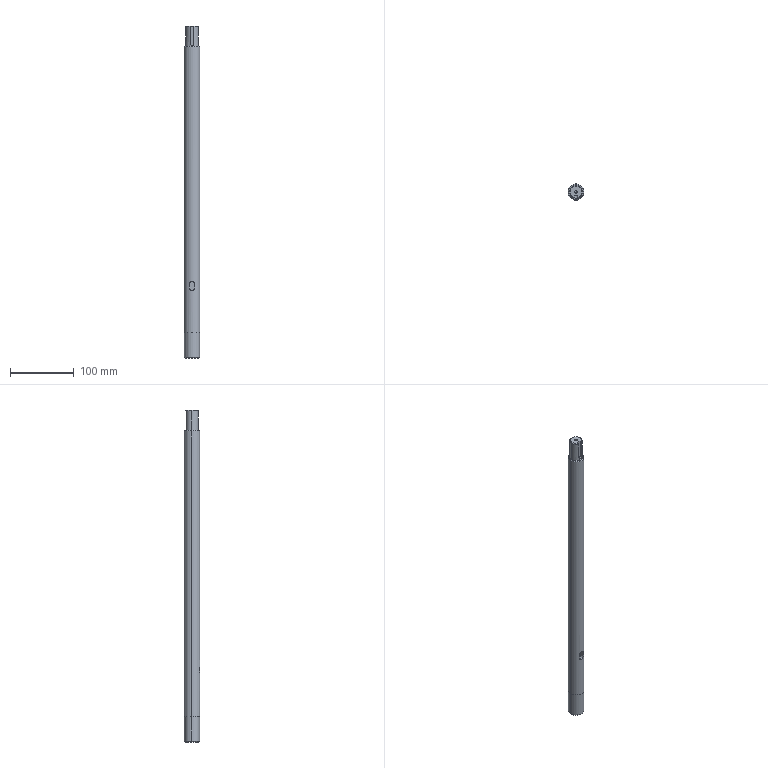Part | SolidWorks | features ICE 4, Chamfer 1, Extrusion 1, Fillet 1, HoleWzd 1 | 1 solid | 32 faces | box 25 x 25 x 522 mm | volume 247598 mm3 | cylinder 13 | plane 10 | cone 9 | commonest cylinder face diameters 8 x4 4.2 x2 20 x2 24 x2 25 x2 6 x1
STEP:
#1=CARTESIAN_POINT('',(-2.1,0.,244.6));
#2=VERTEX_POINT('',#1);
#3=CARTESIAN_POINT('',(2.1,0.,244.6));
#4=VERTEX_POINT('',#3);
#5=CARTESIAN_POINT('',(0.,0.,244.6));
#6=DIRECTION('',(0.,0.,1.));
#7=DIRECTION('',(1.,0.,0.));
#8=AXIS2_PLACEMENT_3D('',#5,#6,#7);
#9=CIRCLE('',#8,2.1);
#10=EDGE_CURVE('',#2,#4,#9,.T.);
#11=ORIENTED_EDGE('',*,*,#10,.F.);
#12=CARTESIAN_POINT('',(-2.1,0.,257.));
#13=VERTEX_POINT('',#12);
#14=CARTESIAN_POINT('',(-2.1,0.,257.));
#15=DIRECTION('',(0.,0.,1.));
#16=VECTOR('',#15,1000.);
#17=LINE('',#14,#16);
#18=EDGE_CURVE('',#2,#13,#17,.T.);
#19=ORIENTED_EDGE('',*,*,#18,.T.);
#20=CARTESIAN_POINT('',(2.1,0.,257.));
#21=VERTEX_POINT('',#20);
#22=CARTESIAN_POINT('',(0.,0.,257.));
#23=DIRECTION('',(0.,0.,1.));
#24=DIRECTION('',(1.,0.,0.));
#25=AXIS2_PLACEMENT_3D('',#22,#23,#24);
#26=CIRCLE('',#25,2.1);
#27=EDGE_CURVE('',#13,#21,#26,.T.);
#28=ORIENTED_EDGE('',*,*,#27,.T.);
#29=CARTESIAN_POINT('',(2.1,0.,257.));
#30=DIRECTION('',(0.,0.,1.));
#31=VECTOR('',#30,1000.);
#32=LINE('',#29,#31);
#33=EDGE_CURVE('',#4,#21,#32,.T.);
#34=ORIENTED_EDGE('',*,*,#33,.F.);
#35=EDGE_LOOP('',(#11,#19,#28,#34));
#36=FACE_OUTER_BOUND('',#35,.T.);
#37=CARTESIAN_POINT('',(0.,0.,257.));
#38=DIRECTION('',(0.,0.,1.));
#39=DIRECTION('',(1.,0.,0.));
#40=AXIS2_PLACEMENT_3D('',#37,#38,#39);
#41=CYLINDRICAL_SURFACE('',#40,2.1);
#42=ADVANCED_FACE('',(#36),#41,.F.);
#43=CARTESIAN_POINT('',(0.,0.,243.338));
#44=VERTEX_POINT('',#43);
#45=CARTESIAN_POINT('',(2.1,0.,244.6));
#46=DIRECTION('',(0.8572,0.,0.515));
#47=VECTOR('',#46,1000.);
#48=LINE('',#45,#47);
#49=EDGE_CURVE('',#44,#4,#48,.T.);
#50=ORIENTED_EDGE('',*,*,#49,.F.);
#51=CARTESIAN_POINT('',(-2.1,0.,244.6));
#52=DIRECTION('',(-0.8572,0.,0.515));
#53=VECTOR('',#52,1000.);
#54=LINE('',#51,#53);
#55=EDGE_CURVE('',#44,#2,#54,.T.);
#56=ORIENTED_EDGE('',*,*,#55,.T.);
#57=ORIENTED_EDGE('',*,*,#10,.T.);
#58=EDGE_LOOP('',(#50,#56,#57));
#59=FACE_OUTER_BOUND('',#58,.T.);
#60=CARTESIAN_POINT('',(0.,0.,244.6));
#61=DIRECTION('',(0.,0.,1.));
#62=DIRECTION('',(1.,0.,0.));
#63=AXIS2_PLACEMENT_3D('',#60,#61,#62);
#64=CONICAL_SURFACE('',#63,2.1,1.03);
#65=ADVANCED_FACE('',(#59),#64,.F.);
#66=CARTESIAN_POINT('',(-11.,0.,-265.));
#67=VERTEX_POINT('',#66);
#68=CARTESIAN_POINT('',(11.,0.,-265.));
#69=VERTEX_POINT('',#68);
#70=CARTESIAN_POINT('',(0.,0.,-265.));
#71=DIRECTION('',(0.,0.,-1.));
#72=DIRECTION('',(-1.,0.,0.));
#73=AXIS2_PLACEMENT_3D('',#70,#71,#72);
#74=CIRCLE('',#73,11.);
#75=EDGE_CURVE('',#67,#69,#74,.T.);
#76=ORIENTED_EDGE('',*,*,#75,.F.);
#77=CARTESIAN_POINT('',(-12.,0.,-264.));
#78=VERTEX_POINT('',#77);
#79=CARTESIAN_POINT('',(-11.,0.,-265.));
#80=DIRECTION('',(-0.7071,0.,0.7071));
#81=VECTOR('',#80,1000.);
#82=LINE('',#79,#81);
#83=EDGE_CURVE('',#67,#78,#82,.T.);
#84=ORIENTED_EDGE('',*,*,#83,.T.);
#85=CARTESIAN_POINT('',(12.,0.,-264.));
#86=VERTEX_POINT('',#85);
#87=CARTESIAN_POINT('',(0.,0.,-264.));
#88=DIRECTION('',(0.,0.,1.));
#89=DIRECTION('',(-1.,0.,0.));
#90=AXIS2_PLACEMENT_3D('',#87,#88,#89);
#91=CIRCLE('',#90,12.);
#92=EDGE_CURVE('',#86,#78,#91,.T.);
#93=ORIENTED_EDGE('',*,*,#92,.F.);
#94=CARTESIAN_POINT('',(11.,0.,-265.));
#95=DIRECTION('',(0.7071,0.,0.7071));
#96=VECTOR('',#95,1000.);
#97=LINE('',#94,#96);
#98=EDGE_CURVE('',#69,#86,#97,.T.);
#99=ORIENTED_EDGE('',*,*,#98,.F.);
#100=EDGE_LOOP('',(#76,#84,#93,#99));
#101=FACE_OUTER_BOUND('',#100,.T.);
#102=CARTESIAN_POINT('',(0.,0.,-265.));
#103=DIRECTION('',(0.,0.,1.));
#104=DIRECTION('',(1.,0.,0.));
#105=AXIS2_PLACEMENT_3D('',#102,#103,#104);
#106=CONICAL_SURFACE('',#105,11.,0.7854);
#107=ADVANCED_FACE('',(#101),#106,.T.);
#108=CARTESIAN_POINT('',(11.5,0.,225.));
#109=VERTEX_POINT('',#108);
#110=CARTESIAN_POINT('',(-11.5,0.,225.));
#111=VERTEX_POINT('',#110);
#112=CARTESIAN_POINT('',(0.,0.,225.));
#113=DIRECTION('',(0.,0.,1.));
#114=DIRECTION('',(1.,0.,0.));
#115=AXIS2_PLACEMENT_3D('',#112,#113,#114);
#116=CIRCLE('',#115,11.5);
#117=EDGE_CURVE('',#109,#111,#116,.T.);
#118=ORIENTED_EDGE('',*,*,#117,.F.);
#119=CARTESIAN_POINT('',(12.5,0.,224.));
#120=VERTEX_POINT('',#119);
#121=CARTESIAN_POINT('',(11.5,0.,225.));
#122=DIRECTION('',(0.7071,0.,-0.7071));
#123=VECTOR('',#122,1000.);
#124=LINE('',#121,#123);
#125=EDGE_CURVE('',#109,#120,#124,.T.);
#126=ORIENTED_EDGE('',*,*,#125,.T.);
#127=CARTESIAN_POINT('',(-12.5,0.,224.));
#128=VERTEX_POINT('',#127);
#129=CARTESIAN_POINT('',(0.,0.,224.));
#130=DIRECTION('',(0.,0.,-1.));
#131=DIRECTION('',(1.,0.,0.));
#132=AXIS2_PLACEMENT_3D('',#129,#130,#131);
#133=CIRCLE('',#132,12.5);
#134=EDGE_CURVE('',#128,#120,#133,.T.);
#135=ORIENTED_EDGE('',*,*,#134,.F.);
#136=CARTESIAN_POINT('',(-11.5,0.,225.));
#137=DIRECTION('',(-0.7071,0.,-0.7071));
#138=VECTOR('',#137,1000.);
#139=LINE('',#136,#138);
#140=EDGE_CURVE('',#111,#128,#139,.T.);
#141=ORIENTED_EDGE('',*,*,#140,.F.);
#142=EDGE_LOOP('',(#118,#126,#135,#141));
#143=FACE_OUTER_BOUND('',#142,.T.);
#144=CARTESIAN_POINT('',(0.,0.,225.));
#145=DIRECTION('',(0.,0.,-1.));
#146=DIRECTION('',(-1.,0.,0.));
#147=AXIS2_PLACEMENT_3D('',#144,#145,#146);
#148=CONICAL_SURFACE('',#147,11.5,0.7854);
#149=ADVANCED_FACE('',(#143),#148,.T.);
#150=CARTESIAN_POINT('',(9.,0.,257.));
#151=VERTEX_POINT('',#150);
#152=CARTESIAN_POINT('',(-9.,0.,257.));
#153=VERTEX_POINT('',#152);
#154=CARTESIAN_POINT('',(0.,0.,257.));
#155=DIRECTION('',(0.,0.,1.));
#156=DIRECTION('',(1.,0.,0.));
#157=AXIS2_PLACEMENT_3D('',#154,#155,#156);
#158=CIRCLE('',#157,9.);
#159=EDGE_CURVE('',#151,#153,#158,.T.);
#160=ORIENTED_EDGE('',*,*,#159,.F.);
#161=CARTESIAN_POINT('',(10.,0.,256.));
#162=VERTEX_POINT('',#161);
#163=CARTESIAN_POINT('',(9.,0.,257.));
#164=DIRECTION('',(0.7071,0.,-0.7071));
#165=VECTOR('',#164,1000.);
#166=LINE('',#163,#165);
#167=EDGE_CURVE('',#151,#162,#166,.T.);
#168=ORIENTED_EDGE('',*,*,#167,.T.);
#169=CARTESIAN_POINT('',(-10.,0.,256.));
#170=VERTEX_POINT('',#169);
#171=CARTESIAN_POINT('',(0.,0.,256.));
#172=DIRECTION('',(0.,0.,-1.));
#173=DIRECTION('',(1.,0.,0.));
#174=AXIS2_PLACEMENT_3D('',#171,#172,#173);
#175=CIRCLE('',#174,10.);
#176=EDGE_CURVE('',#170,#162,#175,.T.);
#177=ORIENTED_EDGE('',*,*,#176,.F.);
#178=CARTESIAN_POINT('',(-9.,0.,257.));
#179=DIRECTION('',(-0.7071,0.,-0.7071));
#180=VECTOR('',#179,1000.);
#181=LINE('',#178,#180);
#182=EDGE_CURVE('',#153,#170,#181,.T.);
#183=ORIENTED_EDGE('',*,*,#182,.F.);
#184=EDGE_LOOP('',(#160,#168,#177,#183));
#185=FACE_OUTER_BOUND('',#184,.T.);
#186=CARTESIAN_POINT('',(0.,0.,257.));
#187=DIRECTION('',(0.,0.,-1.));
#188=DIRECTION('',(-1.,0.,0.));
#189=AXIS2_PLACEMENT_3D('',#186,#187,#188);
#190=CONICAL_SURFACE('',#189,9.,0.7854);
#191=ADVANCED_FACE('',(#185),#190,.T.);
#192=CARTESIAN_POINT('',(-3.,-8.485,257.));
#193=VERTEX_POINT('',#192);
#194=CARTESIAN_POINT('',(0.,0.,257.));
#195=DIRECTION('',(0.,0.,1.));
#196=DIRECTION('',(1.,0.,0.));
#197=AXIS2_PLACEMENT_3D('',#194,#195,#196);
#198=CIRCLE('',#197,9.);
#199=EDGE_CURVE('',#153,#193,#198,.T.);
#200=ORIENTED_EDGE('',*,*,#199,.F.);
#201=ORIENTED_EDGE('',*,*,#182,.T.);
#202=CARTESIAN_POINT('',(-3.,-9.539,256.));
#203=VERTEX_POINT('',#202);
#204=CARTESIAN_POINT('',(0.,0.,256.));
#205=DIRECTION('',(0.,0.,-1.));
#206=DIRECTION('',(1.,0.,0.));
#207=AXIS2_PLACEMENT_3D('',#204,#205,#206);
#208=CIRCLE('',#207,10.);
#209=EDGE_CURVE('',#203,#170,#208,.T.);
#210=ORIENTED_EDGE('',*,*,#209,.F.);
#211=CARTESIAN_POINT('',(-3.,-8.485,257.));
#212=CARTESIAN_POINT('',(-3.,-8.838,256.668));
#213=CARTESIAN_POINT('',(-3.,-9.189,256.334));
#214=CARTESIAN_POINT('',(-3.,-9.539,256.));
#215=B_SPLINE_CURVE_WITH_KNOTS('',3,(#211,#212,#213,#214),.UNSPECIFIED.,.F.,.F.,(4,4),(0.,0.001453),.UNSPECIFIED.);
#216=EDGE_CURVE('',#193,#203,#215,.T.);
#217=ORIENTED_EDGE('',*,*,#216,.F.);
#218=EDGE_LOOP('',(#200,#201,#210,#217));
#219=FACE_OUTER_BOUND('',#218,.T.);
#220=CARTESIAN_POINT('',(0.,0.,257.));
#221=DIRECTION('',(0.,0.,-1.));
#222=DIRECTION('',(-1.,0.,0.));
#223=AXIS2_PLACEMENT_3D('',#220,#221,#222);
#224=CONICAL_SURFACE('',#223,9.,0.7854);
#225=ADVANCED_FACE('',(#219),#224,.T.);
#226=ORIENTED_EDGE('',*,*,#92,.T.);
#227=CARTESIAN_POINT('',(-12.,0.,-225.));
#228=VERTEX_POINT('',#227);
#229=CARTESIAN_POINT('',(-12.,0.,-265.));
#230=DIRECTION('',(0.,0.,1.));
#231=VECTOR('',#230,1000.);
#232=LINE('',#229,#231);
#233=EDGE_CURVE('',#78,#228,#232,.T.);
#234=ORIENTED_EDGE('',*,*,#233,.T.);
#235=CARTESIAN_POINT('',(12.,0.,-225.));
#236=VERTEX_POINT('',#235);
#237=CARTESIAN_POINT('',(0.,0.,-225.));
#238=DIRECTION('',(0.,0.,-1.));
#239=DIRECTION('',(-1.,0.,0.));
#240=AXIS2_PLACEMENT_3D('',#237,#238,#239);
#241=CIRCLE('',#240,12.);
#242=EDGE_CURVE('',#228,#236,#241,.T.);
#243=ORIENTED_EDGE('',*,*,#242,.T.);
#244=CARTESIAN_POINT('',(12.,0.,-265.));
#245=DIRECTION('',(0.,0.,1.));
#246=VECTOR('',#245,1000.);
#247=LINE('',#244,#246);
#248=EDGE_CURVE('',#86,#236,#247,.T.);
#249=ORIENTED_EDGE('',*,*,#248,.F.);
#250=EDGE_LOOP('',(#226,#234,#243,#249));
#251=FACE_OUTER_BOUND('',#250,.T.);
#252=CARTESIAN_POINT('',(0.,0.,-265.));
#253=DIRECTION('',(0.,0.,1.));
#254=DIRECTION('',(1.,0.,0.));
#255=AXIS2_PLACEMENT_3D('',#252,#253,#254);
#256=CYLINDRICAL_SURFACE('',#255,12.);
#257=ADVANCED_FACE('',(#251),#256,.T.);
#258=ORIENTED_EDGE('',*,*,#176,.T.);
#259=CARTESIAN_POINT('',(10.,0.,225.));
#260=VERTEX_POINT('',#259);
#261=CARTESIAN_POINT('',(10.,0.,257.));
#262=DIRECTION('',(0.,0.,-1.));
#263=VECTOR('',#262,1000.);
#264=LINE('',#261,#263);
#265=EDGE_CURVE('',#162,#260,#264,.T.);
#266=ORIENTED_EDGE('',*,*,#265,.T.);
#267=CARTESIAN_POINT('',(-10.,0.,225.));
#268=VERTEX_POINT('',#267);
#269=CARTESIAN_POINT('',(0.,0.,225.));
#270=DIRECTION('',(0.,0.,1.));
#271=DIRECTION('',(1.,0.,0.));
#272=AXIS2_PLACEMENT_3D('',#269,#270,#271);
#273=CIRCLE('',#272,10.);
#274=EDGE_CURVE('',#260,#268,#273,.T.);
#275=ORIENTED_EDGE('',*,*,#274,.T.);
#276=CARTESIAN_POINT('',(-10.,0.,257.));
#277=DIRECTION('',(0.,0.,-1.));
#278=VECTOR('',#277,1000.);
#279=LINE('',#276,#278);
#280=EDGE_CURVE('',#170,#268,#279,.T.);
#281=ORIENTED_EDGE('',*,*,#280,.F.);
#282=EDGE_LOOP('',(#258,#266,#275,#281));
#283=FACE_OUTER_BOUND('',#282,.T.);
#284=CARTESIAN_POINT('',(0.,0.,257.));
#285=DIRECTION('',(0.,0.,-1.));
#286=DIRECTION('',(-1.,0.,0.));
#287=AXIS2_PLACEMENT_3D('',#284,#285,#286);
#288=CYLINDRICAL_SURFACE('',#287,10.);
#289=ADVANCED_FACE('',(#283),#288,.T.);
#290=ORIENTED_EDGE('',*,*,#134,.T.);
#291=CARTESIAN_POINT('',(12.5,0.,-225.));
#292=VERTEX_POINT('',#291);
#293=CARTESIAN_POINT('',(12.5,0.,225.));
#294=DIRECTION('',(0.,0.,-1.));
#295=VECTOR('',#294,1000.);
#296=LINE('',#293,#295);
#297=EDGE_CURVE('',#120,#292,#296,.T.);
#298=ORIENTED_EDGE('',*,*,#297,.T.);
#299=CARTESIAN_POINT('',(-12.5,0.,-225.));
#300=VERTEX_POINT('',#299);
#301=CARTESIAN_POINT('',(0.,0.,-225.));
#302=DIRECTION('',(0.,0.,1.));
#303=DIRECTION('',(1.,0.,0.));
#304=AXIS2_PLACEMENT_3D('',#301,#302,#303);
#305=CIRCLE('',#304,12.5);
#306=EDGE_CURVE('',#292,#300,#305,.T.);
#307=ORIENTED_EDGE('',*,*,#306,.T.);
#308=CARTESIAN_POINT('',(-12.5,0.,225.));
#309=DIRECTION('',(0.,0.,-1.));
#310=VECTOR('',#309,1000.);
#311=LINE('',#308,#310);
#312=EDGE_CURVE('',#128,#300,#311,.T.);
#313=ORIENTED_EDGE('',*,*,#312,.F.);
#314=EDGE_LOOP('',(#290,#298,#307,#313));
#315=FACE_OUTER_BOUND('',#314,.T.);
#316=CARTESIAN_POINT('',(0.,0.,225.));
#317=DIRECTION('',(0.,0.,-1.));
#318=DIRECTION('',(-1.,0.,0.));
#319=AXIS2_PLACEMENT_3D('',#316,#317,#318);
#320=CYLINDRICAL_SURFACE('',#319,12.5);
#321=ADVANCED_FACE('',(#315),#320,.T.);
#322=ORIENTED_EDGE('',*,*,#297,.F.);
#323=CARTESIAN_POINT('',(0.,0.,224.));
#324=DIRECTION('',(0.,0.,-1.));
#325=DIRECTION('',(1.,0.,0.));
#326=AXIS2_PLACEMENT_3D('',#323,#324,#325);
#327=CIRCLE('',#326,12.5);
#328=EDGE_CURVE('',#120,#128,#327,.T.);
#329=ORIENTED_EDGE('',*,*,#328,.T.);
#330=ORIENTED_EDGE('',*,*,#312,.T.);
#331=CARTESIAN_POINT('',(0.,0.,-225.));
#332=DIRECTION('',(0.,0.,1.));
#333=DIRECTION('',(1.,0.,0.));
#334=AXIS2_PLACEMENT_3D('',#331,#332,#333);
#335=CIRCLE('',#334,12.5);
#336=EDGE_CURVE('',#300,#292,#335,.T.);
#337=ORIENTED_EDGE('',*,*,#336,.T.);
#338=EDGE_LOOP('',(#322,#329,#330,#337));
#339=FACE_OUTER_BOUND('',#338,.T.);
#340=CARTESIAN_POINT('',(4.,-11.843,-155.));
#341=VERTEX_POINT('',#340);
#342=CARTESIAN_POINT('',(0.,-12.5,-159.));
#343=VERTEX_POINT('',#342);
#344=CARTESIAN_POINT('',(4.,-11.843,-155.));
#345=CARTESIAN_POINT('',(4.,-11.843,-155.266));
#346=CARTESIAN_POINT('',(3.974,-11.852,-155.527));
#347=CARTESIAN_POINT('',(3.871,-11.886,-156.04));
#348=CARTESIAN_POINT('',(3.794,-11.911,-156.295));
#349=CARTESIAN_POINT('',(3.592,-11.973,-156.779));
#350=CARTESIAN_POINT('',(3.47,-12.01,-157.007));
#351=CARTESIAN_POINT('',(3.18,-12.09,-157.441));
#352=CARTESIAN_POINT('',(3.012,-12.133,-157.644));
#353=CARTESIAN_POINT('',(2.646,-12.218,-158.011));
#354=CARTESIAN_POINT('',(2.446,-12.26,-158.176));
#355=CARTESIAN_POINT('',(2.01,-12.339,-158.468));
#356=CARTESIAN_POINT('',(1.78,-12.375,-158.591));
#357=CARTESIAN_POINT('',(1.3,-12.435,-158.792));
#358=CARTESIAN_POINT('',(1.047,-12.459,-158.87));
#359=CARTESIAN_POINT('',(0.5285,-12.492,-158.974));
#360=CARTESIAN_POINT('',(0.266,-12.5,-159.));
#361=CARTESIAN_POINT('',(0.,-12.5,-159.));
#362=B_SPLINE_CURVE_WITH_KNOTS('',3,(#344,#345,#346,#347,#348,#349,#350,#351,#352,#353,#354,#355,#356,#357,#358,#359,#360,#361),.UNSPECIFIED.,.F.,.F.,(4,2,2,2,2,2,2,2,4),(0.,0.0007863,0.001573,0.002359,0.003145,0.003931,0.004718,0.005504,0.00629),.UNSPECIFIED.);
#363=EDGE_CURVE('',#341,#343,#362,.T.);
#364=ORIENTED_EDGE('',*,*,#363,.T.);
#365=CARTESIAN_POINT('',(-4.,-11.843,-155.));
#366=VERTEX_POINT('',#365);
#367=CARTESIAN_POINT('',(0.,-12.5,-159.));
#368=CARTESIAN_POINT('',(-0.266,-12.5,-159.));
#369=CARTESIAN_POINT('',(-0.5272,-12.492,-158.974));
#370=CARTESIAN_POINT('',(-1.041,-12.459,-158.871));
#371=CARTESIAN_POINT('',(-1.296,-12.435,-158.793));
#372=CARTESIAN_POINT('',(-1.779,-12.375,-158.592));
#373=CARTESIAN_POINT('',(-2.008,-12.34,-158.469));
#374=CARTESIAN_POINT('',(-2.441,-12.261,-158.179));
#375=CARTESIAN_POINT('',(-2.645,-12.218,-158.012));
#376=CARTESIAN_POINT('',(-3.011,-12.133,-157.646));
#377=CARTESIAN_POINT('',(-3.176,-12.091,-157.446));
#378=CARTESIAN_POINT('',(-3.469,-12.01,-157.009));
#379=CARTESIAN_POINT('',(-3.592,-11.973,-156.78));
#380=CARTESIAN_POINT('',(-3.792,-11.911,-156.3));
#381=CARTESIAN_POINT('',(-3.87,-11.886,-156.046));
#382=CARTESIAN_POINT('',(-3.974,-11.852,-155.528));
#383=CARTESIAN_POINT('',(-4.,-11.843,-155.266));
#384=CARTESIAN_POINT('',(-4.,-11.843,-155.));
#385=B_SPLINE_CURVE_WITH_KNOTS('',3,(#367,#368,#369,#370,#371,#372,#373,#374,#375,#376,#377,#378,#379,#380,#381,#382,#383,#384),.UNSPECIFIED.,.F.,.F.,(4,2,2,2,2,2,2,2,4),(0.,0.0007863,0.001573,0.002359,0.003145,0.003932,0.004718,0.005504,0.00629),.UNSPECIFIED.);
#386=EDGE_CURVE('',#343,#366,#385,.T.);
#387=ORIENTED_EDGE('',*,*,#386,.T.);
#388=CARTESIAN_POINT('',(-4.,-11.843,-148.));
#389=VERTEX_POINT('',#388);
#390=CARTESIAN_POINT('',(-4.,-11.843,225.));
#391=DIRECTION('',(0.,0.,1.));
#392=VECTOR('',#391,1000.);
#393=LINE('',#390,#392);
#394=EDGE_CURVE('',#366,#389,#393,.T.);
#395=ORIENTED_EDGE('',*,*,#394,.T.);
#396=CARTESIAN_POINT('',(0.,-12.5,-144.));
#397=VERTEX_POINT('',#396);
#398=CARTESIAN_POINT('',(-4.,-11.843,-148.));
#399=CARTESIAN_POINT('',(-4.,-11.843,-147.734));
#400=CARTESIAN_POINT('',(-3.974,-11.852,-147.473));
#401=CARTESIAN_POINT('',(-3.871,-11.886,-146.96));
#402=CARTESIAN_POINT('',(-3.794,-11.911,-146.705));
#403=CARTESIAN_POINT('',(-3.592,-11.973,-146.221));
#404=CARTESIAN_POINT('',(-3.47,-12.01,-145.993));
#405=CARTESIAN_POINT('',(-3.18,-12.09,-145.559));
#406=CARTESIAN_POINT('',(-3.012,-12.133,-145.356));
#407=CARTESIAN_POINT('',(-2.646,-12.218,-144.989));
#408=CARTESIAN_POINT('',(-2.446,-12.26,-144.824));
#409=CARTESIAN_POINT('',(-2.01,-12.339,-144.532));
#410=CARTESIAN_POINT('',(-1.78,-12.375,-144.409));
#411=CARTESIAN_POINT('',(-1.3,-12.435,-144.208));
#412=CARTESIAN_POINT('',(-1.047,-12.459,-144.13));
#413=CARTESIAN_POINT('',(-0.5285,-12.492,-144.026));
#414=CARTESIAN_POINT('',(-0.266,-12.5,-144.));
#415=CARTESIAN_POINT('',(0.,-12.5,-144.));
#416=B_SPLINE_CURVE_WITH_KNOTS('',3,(#398,#399,#400,#401,#402,#403,#404,#405,#406,#407,#408,#409,#410,#411,#412,#413,#414,#415),.UNSPECIFIED.,.F.,.F.,(4,2,2,2,2,2,2,2,4),(0.,0.0007863,0.001573,0.002359,0.003145,0.003931,0.004718,0.005504,0.00629),.UNSPECIFIED.);
#417=EDGE_CURVE('',#389,#397,#416,.T.);
#418=ORIENTED_EDGE('',*,*,#417,.T.);
#419=CARTESIAN_POINT('',(4.,-11.843,-148.));
#420=VERTEX_POINT('',#419);
#421=CARTESIAN_POINT('',(0.,-12.5,-144.));
#422=CARTESIAN_POINT('',(0.266,-12.5,-144.));
#423=CARTESIAN_POINT('',(0.5272,-12.492,-144.026));
#424=CARTESIAN_POINT('',(1.041,-12.459,-144.129));
#425=CARTESIAN_POINT('',(1.296,-12.435,-144.207));
#426=CARTESIAN_POINT('',(1.779,-12.375,-144.408));
#427=CARTESIAN_POINT('',(2.008,-12.34,-144.531));
#428=CARTESIAN_POINT('',(2.441,-12.261,-144.821));
#429=CARTESIAN_POINT('',(2.645,-12.218,-144.988));
#430=CARTESIAN_POINT('',(3.011,-12.133,-145.354));
#431=CARTESIAN_POINT('',(3.176,-12.091,-145.554));
#432=CARTESIAN_POINT('',(3.469,-12.01,-145.991));
#433=CARTESIAN_POINT('',(3.592,-11.973,-146.22));
#434=CARTESIAN_POINT('',(3.792,-11.911,-146.7));
#435=CARTESIAN_POINT('',(3.87,-11.886,-146.954));
#436=CARTESIAN_POINT('',(3.974,-11.852,-147.472));
#437=CARTESIAN_POINT('',(4.,-11.843,-147.734));
#438=CARTESIAN_POINT('',(4.,-11.843,-148.));
#439=B_SPLINE_CURVE_WITH_KNOTS('',3,(#421,#422,#423,#424,#425,#426,#427,#428,#429,#430,#431,#432,#433,#434,#435,#436,#437,#438),.UNSPECIFIED.,.F.,.F.,(4,2,2,2,2,2,2,2,4),(0.,0.0007863,0.001573,0.002359,0.003145,0.003932,0.004718,0.005504,0.00629),.UNSPECIFIED.);
#440=EDGE_CURVE('',#397,#420,#439,.T.);
#441=ORIENTED_EDGE('',*,*,#440,.T.);
#442=CARTESIAN_POINT('',(4.,-11.843,225.));
#443=DIRECTION('',(0.,0.,-1.));
#444=VECTOR('',#443,1000.);
#445=LINE('',#442,#444);
#446=EDGE_CURVE('',#420,#341,#445,.T.);
#447=ORIENTED_EDGE('',*,*,#446,.T.);
#448=EDGE_LOOP('',(#364,#387,#395,#418,#441,#447));
#449=FACE_BOUND('',#448,.T.);
#450=CARTESIAN_POINT('',(0.,0.,225.));
#451=DIRECTION('',(0.,0.,-1.));
#452=DIRECTION('',(-1.,0.,0.));
#453=AXIS2_PLACEMENT_3D('',#450,#451,#452);
#454=CYLINDRICAL_SURFACE('',#453,12.5);
#455=ADVANCED_FACE('',(#339,#449),#454,.T.);
#456=CARTESIAN_POINT('',(0.,0.,225.));
#457=DIRECTION('',(0.,0.,1.));
#458=DIRECTION('',(1.,0.,0.));
#459=AXIS2_PLACEMENT_3D('',#456,#457,#458);
#460=CIRCLE('',#459,11.5);
#461=EDGE_CURVE('',#111,#109,#460,.T.);
#462=ORIENTED_EDGE('',*,*,#461,.T.);
#463=ORIENTED_EDGE('',*,*,#117,.T.);
#464=EDGE_LOOP('',(#462,#463));
#465=FACE_OUTER_BOUND('',#464,.T.);
#466=CARTESIAN_POINT('',(0.,0.,225.));
#467=DIRECTION('',(0.,0.,1.));
#468=DIRECTION('',(1.,0.,0.));
#469=AXIS2_PLACEMENT_3D('',#466,#467,#468);
#470=CIRCLE('',#469,10.);
#471=EDGE_CURVE('',#268,#260,#470,.T.);
#472=ORIENTED_EDGE('',*,*,#471,.F.);
#473=ORIENTED_EDGE('',*,*,#274,.F.);
#474=EDGE_LOOP('',(#472,#473));
#475=FACE_BOUND('',#474,.T.);
#476=CARTESIAN_POINT('',(0.,0.,225.));
#477=DIRECTION('',(0.,0.,1.));
#478=DIRECTION('',(1.,0.,0.));
#479=AXIS2_PLACEMENT_3D('',#476,#477,#478);
#480=PLANE('',#479);
#481=ADVANCED_FACE('',(#465,#475),#480,.T.);
#482=CARTESIAN_POINT('',(0.,0.,-225.));
#483=DIRECTION('',(0.,0.,-1.));
#484=DIRECTION('',(-1.,0.,0.));
#485=AXIS2_PLACEMENT_3D('',#482,#483,#484);
#486=CIRCLE('',#485,12.);
#487=EDGE_CURVE('',#236,#228,#486,.T.);
#488=ORIENTED_EDGE('',*,*,#487,.F.);
#489=ORIENTED_EDGE('',*,*,#242,.F.);
#490=EDGE_LOOP('',(#488,#489));
#491=FACE_BOUND('',#490,.T.);
#492=ORIENTED_EDGE('',*,*,#336,.F.);
#493=ORIENTED_EDGE('',*,*,#306,.F.);
#494=EDGE_LOOP('',(#492,#493));
#495=FACE_OUTER_BOUND('',#494,.T.);
#496=CARTESIAN_POINT('',(0.,0.,-225.));
#497=DIRECTION('',(0.,0.,1.));
#498=DIRECTION('',(1.,0.,0.));
#499=AXIS2_PLACEMENT_3D('',#496,#497,#498);
#500=PLANE('',#499);
#501=ADVANCED_FACE('',(#491,#495),#500,.F.);
#502=ORIENTED_EDGE('',*,*,#265,.F.);
#503=CARTESIAN_POINT('',(3.,-9.539,256.));
#504=VERTEX_POINT('',#503);
#505=CARTESIAN_POINT('',(0.,0.,256.));
#506=DIRECTION('',(0.,0.,-1.));
#507=DIRECTION('',(1.,0.,0.));
#508=AXIS2_PLACEMENT_3D('',#505,#506,#507);
#509=CIRCLE('',#508,10.);
#510=EDGE_CURVE('',#162,#504,#509,.T.);
#511=ORIENTED_EDGE('',*,*,#510,.T.);
#512=CARTESIAN_POINT('',(3.,-9.539,229.5));
#513=VERTEX_POINT('',#512);
#514=CARTESIAN_POINT('',(3.,-9.539,257.));
#515=DIRECTION('',(0.,0.,-1.));
#516=VECTOR('',#515,1000.);
#517=LINE('',#514,#516);
#518=EDGE_CURVE('',#504,#513,#517,.T.);
#519=ORIENTED_EDGE('',*,*,#518,.T.);
#520=CARTESIAN_POINT('',(-3.,-9.539,229.5));
#521=VERTEX_POINT('',#520);
#522=CARTESIAN_POINT('',(3.,-9.539,229.5));
#523=CARTESIAN_POINT('',(3.,-9.539,229.301));
#524=CARTESIAN_POINT('',(2.98,-9.546,229.105));
#525=CARTESIAN_POINT('',(2.903,-9.569,228.72));
#526=CARTESIAN_POINT('',(2.845,-9.587,228.529));
#527=CARTESIAN_POINT('',(2.694,-9.631,228.166));
#528=CARTESIAN_POINT('',(2.602,-9.656,227.994));
#529=CARTESIAN_POINT('',(2.385,-9.712,227.669));
#530=CARTESIAN_POINT('',(2.259,-9.743,227.516));
#531=CARTESIAN_POINT('',(1.847,-9.832,227.104));
#532=CARTESIAN_POINT('',(1.514,-9.891,226.881));
#533=CARTESIAN_POINT('',(0.9732,-9.954,226.656));
#534=CARTESIAN_POINT('',(0.783,-9.971,226.597));
#535=CARTESIAN_POINT('',(0.3953,-9.994,226.52));
#536=CARTESIAN_POINT('',(0.1999,-10.,226.5));
#537=CARTESIAN_POINT('',(-0.194,-10.,226.5));
#538=CARTESIAN_POINT('',(-0.394,-9.994,226.519));
#539=CARTESIAN_POINT('',(-0.7797,-9.971,226.596));
#540=CARTESIAN_POINT('',(-0.9673,-9.955,226.653));
#541=CARTESIAN_POINT('',(-1.332,-9.913,226.805));
#542=CARTESIAN_POINT('',(-1.506,-9.887,226.898));
#543=CARTESIAN_POINT('',(-1.83,-9.833,227.114));
#544=CARTESIAN_POINT('',(-1.982,-9.803,227.24));
#545=CARTESIAN_POINT('',(-2.259,-9.743,227.516));
#546=CARTESIAN_POINT('',(-2.383,-9.713,227.667));
#547=CARTESIAN_POINT('',(-2.6,-9.657,227.99));
#548=CARTESIAN_POINT('',(-2.694,-9.631,228.166));
#549=CARTESIAN_POINT('',(-2.845,-9.587,228.527));
#550=CARTESIAN_POINT('',(-2.902,-9.57,228.714));
#551=CARTESIAN_POINT('',(-2.98,-9.546,229.101));
#552=CARTESIAN_POINT('',(-3.,-9.539,229.301));
#553=CARTESIAN_POINT('',(-3.,-9.539,229.5));
#554=B_SPLINE_CURVE_WITH_KNOTS('',3,(#522,#523,#524,#525,#526,#527,#528,#529,#530,#531,#532,#533,#534,#535,#536,#537,#538,#539,#540,#541,#542,#543,#544,#545,#546,#547,#548,#549,#550,#551,#552,#553),.UNSPECIFIED.,.F.,.F.,(4,2,2,2,2,2,2,2,2,2,2,2,2,2,2,4),(0.,0.0005894,0.001179,0.001768,0.002358,0.003536,0.004126,0.004715,0.005305,0.005894,0.006484,0.007073,0.007662,0.008252,0.008841,0.009431),.UNSPECIFIED.);
#555=EDGE_CURVE('',#513,#521,#554,.T.);
#556=ORIENTED_EDGE('',*,*,#555,.T.);
#557=CARTESIAN_POINT('',(-3.,-9.539,257.));
#558=DIRECTION('',(0.,0.,1.));
#559=VECTOR('',#558,1000.);
#560=LINE('',#557,#559);
#561=EDGE_CURVE('',#521,#203,#560,.T.);
#562=ORIENTED_EDGE('',*,*,#561,.T.);
#563=ORIENTED_EDGE('',*,*,#209,.T.);
#564=ORIENTED_EDGE('',*,*,#280,.T.);
#565=ORIENTED_EDGE('',*,*,#471,.T.);
#566=EDGE_LOOP('',(#502,#511,#519,#556,#562,#563,#564,#565));
#567=FACE_OUTER_BOUND('',#566,.T.);
#568=CARTESIAN_POINT('',(0.,0.,257.));
#569=DIRECTION('',(0.,0.,-1.));
#570=DIRECTION('',(-1.,0.,0.));
#571=AXIS2_PLACEMENT_3D('',#568,#569,#570);
#572=CYLINDRICAL_SURFACE('',#571,10.);
#573=ADVANCED_FACE('',(#567),#572,.T.);
#574=CARTESIAN_POINT('',(0.,0.,257.));
#575=DIRECTION('',(0.,0.,1.));
#576=DIRECTION('',(1.,0.,0.));
#577=AXIS2_PLACEMENT_3D('',#574,#575,#576);
#578=CIRCLE('',#577,2.1);
#579=EDGE_CURVE('',#21,#13,#578,.T.);
#580=ORIENTED_EDGE('',*,*,#579,.F.);
#581=ORIENTED_EDGE('',*,*,#27,.F.);
#582=EDGE_LOOP('',(#580,#581));
#583=FACE_BOUND('',#582,.T.);
#584=CARTESIAN_POINT('',(3.,-8.485,257.));
#585=VERTEX_POINT('',#584);
#586=CARTESIAN_POINT('',(3.,-6.5,257.));
#587=VERTEX_POINT('',#586);
#588=CARTESIAN_POINT('',(3.,0.,257.));
#589=DIRECTION('',(0.,1.,0.));
#590=VECTOR('',#589,1000.);
#591=LINE('',#588,#590);
#592=EDGE_CURVE('',#585,#587,#591,.T.);
#593=ORIENTED_EDGE('',*,*,#592,.F.);
#594=CARTESIAN_POINT('',(0.,0.,257.));
#595=DIRECTION('',(0.,0.,1.));
#596=DIRECTION('',(1.,0.,0.));
#597=AXIS2_PLACEMENT_3D('',#594,#595,#596);
#598=CIRCLE('',#597,9.);
#599=EDGE_CURVE('',#585,#151,#598,.T.);
#600=ORIENTED_EDGE('',*,*,#599,.T.);
#601=ORIENTED_EDGE('',*,*,#159,.T.);
#602=ORIENTED_EDGE('',*,*,#199,.T.);
#603=CARTESIAN_POINT('',(-3.,-6.5,257.));
#604=VERTEX_POINT('',#603);
#605=CARTESIAN_POINT('',(-3.,0.,257.));
#606=DIRECTION('',(0.,-1.,0.));
#607=VECTOR('',#606,1000.);
#608=LINE('',#605,#607);
#609=EDGE_CURVE('',#604,#193,#608,.T.);
#610=ORIENTED_EDGE('',*,*,#609,.F.);
#611=CARTESIAN_POINT('',(0.,-6.5,257.));
#612=DIRECTION('',(-1.,0.,0.));
#613=VECTOR('',#612,1000.);
#614=LINE('',#611,#613);
#615=EDGE_CURVE('',#587,#604,#614,.T.);
#616=ORIENTED_EDGE('',*,*,#615,.F.);
#617=EDGE_LOOP('',(#593,#600,#601,#602,#610,#616));
#618=FACE_OUTER_BOUND('',#617,.T.);
#619=CARTESIAN_POINT('',(0.,0.,257.));
#620=DIRECTION('',(0.,0.,1.));
#621=DIRECTION('',(1.,0.,0.));
#622=AXIS2_PLACEMENT_3D('',#619,#620,#621);
#623=PLANE('',#622);
#624=ADVANCED_FACE('',(#583,#618),#623,.T.);
#625=CARTESIAN_POINT('',(3.,-6.5,229.5));
#626=VERTEX_POINT('',#625);
#627=CARTESIAN_POINT('',(3.,-16.5,229.5));
#628=DIRECTION('',(0.,1.,0.));
#629=VECTOR('',#628,1000.);
#630=LINE('',#627,#629);
#631=EDGE_CURVE('',#513,#626,#630,.T.);
#632=ORIENTED_EDGE('',*,*,#631,.T.);
#633=CARTESIAN_POINT('',(-3.,-6.5,229.5));
#634=VERTEX_POINT('',#633);
#635=CARTESIAN_POINT('',(0.,-6.5,229.5));
#636=DIRECTION('',(0.,1.,0.));
#637=DIRECTION('',(0.,0.,1.));
#638=AXIS2_PLACEMENT_3D('',#635,#636,#637);
#639=CIRCLE('',#638,3.);
#640=EDGE_CURVE('',#626,#634,#639,.T.);
#641=ORIENTED_EDGE('',*,*,#640,.T.);
#642=CARTESIAN_POINT('',(-3.,-16.5,229.5));
#643=DIRECTION('',(0.,1.,0.));
#644=VECTOR('',#643,1000.);
#645=LINE('',#642,#644);
#646=EDGE_CURVE('',#521,#634,#645,.T.);
#647=ORIENTED_EDGE('',*,*,#646,.F.);
#648=ORIENTED_EDGE('',*,*,#555,.F.);
#649=EDGE_LOOP('',(#632,#641,#647,#648));
#650=FACE_OUTER_BOUND('',#649,.T.);
#651=CARTESIAN_POINT('',(0.,-16.5,229.5));
#652=DIRECTION('',(0.,1.,0.));
#653=DIRECTION('',(0.,0.,1.));
#654=AXIS2_PLACEMENT_3D('',#651,#652,#653);
#655=CYLINDRICAL_SURFACE('',#654,3.);
#656=ADVANCED_FACE('',(#650),#655,.F.);
#657=ORIENTED_EDGE('',*,*,#609,.T.);
#658=ORIENTED_EDGE('',*,*,#216,.T.);
#659=ORIENTED_EDGE('',*,*,#561,.F.);
#660=ORIENTED_EDGE('',*,*,#646,.T.);
#661=CARTESIAN_POINT('',(-3.,-6.5,284.5));
#662=DIRECTION('',(0.,0.,1.));
#663=VECTOR('',#662,1000.);
#664=LINE('',#661,#663);
#665=EDGE_CURVE('',#634,#604,#664,.T.);
#666=ORIENTED_EDGE('',*,*,#665,.T.);
#667=EDGE_LOOP('',(#657,#658,#659,#660,#666));
#668=FACE_OUTER_BOUND('',#667,.T.);
#669=CARTESIAN_POINT('',(-3.,-16.5,284.5));
#670=DIRECTION('',(-1.,0.,0.));
#671=DIRECTION('',(0.,0.,1.));
#672=AXIS2_PLACEMENT_3D('',#669,#670,#671);
#673=PLANE('',#672);
#674=ADVANCED_FACE('',(#668),#673,.F.);
#675=ORIENTED_EDGE('',*,*,#518,.F.);
#676=CARTESIAN_POINT('',(3.,-9.539,256.));
#677=CARTESIAN_POINT('',(3.,-9.189,256.334));
#678=CARTESIAN_POINT('',(3.,-8.838,256.668));
#679=CARTESIAN_POINT('',(3.,-8.485,257.));
#680=B_SPLINE_CURVE_WITH_KNOTS('',3,(#676,#677,#678,#679),.UNSPECIFIED.,.F.,.F.,(4,4),(0.,0.001453),.UNSPECIFIED.);
#681=EDGE_CURVE('',#504,#585,#680,.T.);
#682=ORIENTED_EDGE('',*,*,#681,.T.);
#683=ORIENTED_EDGE('',*,*,#592,.T.);
#684=CARTESIAN_POINT('',(3.,-6.5,284.5));
#685=DIRECTION('',(0.,0.,-1.));
#686=VECTOR('',#685,1000.);
#687=LINE('',#684,#686);
#688=EDGE_CURVE('',#587,#626,#687,.T.);
#689=ORIENTED_EDGE('',*,*,#688,.T.);
#690=ORIENTED_EDGE('',*,*,#631,.F.);
#691=EDGE_LOOP('',(#675,#682,#683,#689,#690));
#692=FACE_OUTER_BOUND('',#691,.T.);
#693=CARTESIAN_POINT('',(3.,-16.5,284.5));
#694=DIRECTION('',(1.,0.,0.));
#695=DIRECTION('',(0.,0.,-1.));
#696=AXIS2_PLACEMENT_3D('',#693,#694,#695);
#697=PLANE('',#696);
#698=ADVANCED_FACE('',(#692),#697,.F.);
#699=ORIENTED_EDGE('',*,*,#615,.T.);
#700=ORIENTED_EDGE('',*,*,#665,.F.);
#701=ORIENTED_EDGE('',*,*,#640,.F.);
#702=ORIENTED_EDGE('',*,*,#688,.F.);
#703=EDGE_LOOP('',(#699,#700,#701,#702));
#704=FACE_OUTER_BOUND('',#703,.T.);
#705=CARTESIAN_POINT('',(0.,-6.5,284.5));
#706=DIRECTION('',(0.,1.,0.));
#707=DIRECTION('',(0.,0.,1.));
#708=AXIS2_PLACEMENT_3D('',#705,#706,#707);
#709=PLANE('',#708);
#710=ADVANCED_FACE('',(#704),#709,.F.);
#711=ORIENTED_EDGE('',*,*,#233,.F.);
#712=CARTESIAN_POINT('',(0.,0.,-264.));
#713=DIRECTION('',(0.,0.,1.));
#714=DIRECTION('',(-1.,0.,0.));
#715=AXIS2_PLACEMENT_3D('',#712,#713,#714);
#716=CIRCLE('',#715,12.);
#717=EDGE_CURVE('',#78,#86,#716,.T.);
#718=ORIENTED_EDGE('',*,*,#717,.T.);
#719=ORIENTED_EDGE('',*,*,#248,.T.);
#720=ORIENTED_EDGE('',*,*,#487,.T.);
#721=EDGE_LOOP('',(#711,#718,#719,#720));
#722=FACE_OUTER_BOUND('',#721,.T.);
#723=CARTESIAN_POINT('',(0.,0.,-265.));
#724=DIRECTION('',(0.,0.,1.));
#725=DIRECTION('',(1.,0.,0.));
#726=AXIS2_PLACEMENT_3D('',#723,#724,#725);
#727=CYLINDRICAL_SURFACE('',#726,12.);
#728=ADVANCED_FACE('',(#722),#727,.T.);
#729=CARTESIAN_POINT('',(0.,0.,-265.));
#730=DIRECTION('',(0.,0.,-1.));
#731=DIRECTION('',(-1.,0.,0.));
#732=AXIS2_PLACEMENT_3D('',#729,#730,#731);
#733=CIRCLE('',#732,11.);
#734=EDGE_CURVE('',#69,#67,#733,.T.);
#735=ORIENTED_EDGE('',*,*,#734,.T.);
#736=ORIENTED_EDGE('',*,*,#75,.T.);
#737=EDGE_LOOP('',(#735,#736));
#738=FACE_OUTER_BOUND('',#737,.T.);
#739=CARTESIAN_POINT('',(0.,0.,-265.));
#740=DIRECTION('',(0.,0.,-1.));
#741=DIRECTION('',(-1.,0.,0.));
#742=AXIS2_PLACEMENT_3D('',#739,#740,#741);
#743=PLANE('',#742);
#744=ADVANCED_FACE('',(#738),#743,.T.);
#745=ORIENTED_EDGE('',*,*,#167,.F.);
#746=ORIENTED_EDGE('',*,*,#599,.F.);
#747=ORIENTED_EDGE('',*,*,#681,.F.);
#748=ORIENTED_EDGE('',*,*,#510,.F.);
#749=EDGE_LOOP('',(#745,#746,#747,#748));
#750=FACE_OUTER_BOUND('',#749,.T.);
#751=CARTESIAN_POINT('',(0.,0.,257.));
#752=DIRECTION('',(0.,0.,-1.));
#753=DIRECTION('',(-1.,0.,0.));
#754=AXIS2_PLACEMENT_3D('',#751,#752,#753);
#755=CONICAL_SURFACE('',#754,9.,0.7854);
#756=ADVANCED_FACE('',(#750),#755,.T.);
#757=ORIENTED_EDGE('',*,*,#125,.F.);
#758=ORIENTED_EDGE('',*,*,#461,.F.);
#759=ORIENTED_EDGE('',*,*,#140,.T.);
#760=ORIENTED_EDGE('',*,*,#328,.F.);
#761=EDGE_LOOP('',(#757,#758,#759,#760));
#762=FACE_OUTER_BOUND('',#761,.T.);
#763=CARTESIAN_POINT('',(0.,0.,225.));
#764=DIRECTION('',(0.,0.,-1.));
#765=DIRECTION('',(-1.,0.,0.));
#766=AXIS2_PLACEMENT_3D('',#763,#764,#765);
#767=CONICAL_SURFACE('',#766,11.5,0.7854);
#768=ADVANCED_FACE('',(#762),#767,.T.);
#769=ORIENTED_EDGE('',*,*,#83,.F.);
#770=ORIENTED_EDGE('',*,*,#734,.F.);
#771=ORIENTED_EDGE('',*,*,#98,.T.);
#772=ORIENTED_EDGE('',*,*,#717,.F.);
#773=EDGE_LOOP('',(#769,#770,#771,#772));
#774=FACE_OUTER_BOUND('',#773,.T.);
#775=CARTESIAN_POINT('',(0.,0.,-265.));
#776=DIRECTION('',(0.,0.,1.));
#777=DIRECTION('',(1.,0.,0.));
#778=AXIS2_PLACEMENT_3D('',#775,#776,#777);
#779=CONICAL_SURFACE('',#778,11.,0.7854);
#780=ADVANCED_FACE('',(#774),#779,.T.);
#781=ORIENTED_EDGE('',*,*,#55,.F.);
#782=ORIENTED_EDGE('',*,*,#49,.T.);
#783=CARTESIAN_POINT('',(0.,0.,244.6));
#784=DIRECTION('',(0.,0.,1.));
#785=DIRECTION('',(1.,0.,0.));
#786=AXIS2_PLACEMENT_3D('',#783,#784,#785);
#787=CIRCLE('',#786,2.1);
#788=EDGE_CURVE('',#4,#2,#787,.T.);
#789=ORIENTED_EDGE('',*,*,#788,.T.);
#790=EDGE_LOOP('',(#781,#782,#789));
#791=FACE_OUTER_BOUND('',#790,.T.);
#792=CARTESIAN_POINT('',(0.,0.,244.6));
#793=DIRECTION('',(0.,0.,1.));
#794=DIRECTION('',(1.,0.,0.));
#795=AXIS2_PLACEMENT_3D('',#792,#793,#794);
#796=CONICAL_SURFACE('',#795,2.1,1.03);
#797=ADVANCED_FACE('',(#791),#796,.F.);
#798=ORIENTED_EDGE('',*,*,#18,.F.);
#799=ORIENTED_EDGE('',*,*,#788,.F.);
#800=ORIENTED_EDGE('',*,*,#33,.T.);
#801=ORIENTED_EDGE('',*,*,#579,.T.);
#802=EDGE_LOOP('',(#798,#799,#800,#801));
#803=FACE_OUTER_BOUND('',#802,.T.);
#804=CARTESIAN_POINT('',(0.,0.,257.));
#805=DIRECTION('',(0.,0.,1.));
#806=DIRECTION('',(1.,0.,0.));
#807=AXIS2_PLACEMENT_3D('',#804,#805,#806);
#808=CYLINDRICAL_SURFACE('',#807,2.1);
#809=ADVANCED_FACE('',(#803),#808,.F.);
#810=CARTESIAN_POINT('',(-4.,-7.,-155.));
#811=VERTEX_POINT('',#810);
#812=CARTESIAN_POINT('',(-4.,-7.,-148.));
#813=VERTEX_POINT('',#812);
#814=CARTESIAN_POINT('',(-4.,-7.,-159.));
#815=DIRECTION('',(0.,0.,1.));
#816=VECTOR('',#815,1000.);
#817=LINE('',#814,#816);
#818=EDGE_CURVE('',#811,#813,#817,.T.);
#819=ORIENTED_EDGE('',*,*,#818,.T.);
#820=CARTESIAN_POINT('',(-4.,-11.843,-148.));
#821=DIRECTION('',(0.,-1.,0.));
#822=VECTOR('',#821,1000.);
#823=LINE('',#820,#822);
#824=EDGE_CURVE('',#813,#389,#823,.T.);
#825=ORIENTED_EDGE('',*,*,#824,.T.);
#826=ORIENTED_EDGE('',*,*,#394,.F.);
#827=CARTESIAN_POINT('',(-4.,-7.,-155.));
#828=DIRECTION('',(0.,1.,0.));
#829=VECTOR('',#828,1000.);
#830=LINE('',#827,#829);
#831=EDGE_CURVE('',#366,#811,#830,.T.);
#832=ORIENTED_EDGE('',*,*,#831,.T.);
#833=EDGE_LOOP('',(#819,#825,#826,#832));
#834=FACE_OUTER_BOUND('',#833,.T.);
#835=CARTESIAN_POINT('',(-4.,-7.,-159.));
#836=DIRECTION('',(-1.,0.,0.));
#837=DIRECTION('',(0.,-1.,0.));
#838=AXIS2_PLACEMENT_3D('',#835,#836,#837);
#839=PLANE('',#838);
#840=ADVANCED_FACE('',(#834),#839,.F.);
#841=ORIENTED_EDGE('',*,*,#446,.F.);
#842=CARTESIAN_POINT('',(4.,-7.,-148.));
#843=VERTEX_POINT('',#842);
#844=CARTESIAN_POINT('',(4.,-7.,-148.));
#845=DIRECTION('',(0.,1.,0.));
#846=VECTOR('',#845,1000.);
#847=LINE('',#844,#846);
#848=EDGE_CURVE('',#420,#843,#847,.T.);
#849=ORIENTED_EDGE('',*,*,#848,.T.);
#850=CARTESIAN_POINT('',(4.,-7.,-155.));
#851=VERTEX_POINT('',#850);
#852=CARTESIAN_POINT('',(4.,-7.,-159.));
#853=DIRECTION('',(0.,0.,1.));
#854=VECTOR('',#853,1000.);
#855=LINE('',#852,#854);
#856=EDGE_CURVE('',#851,#843,#855,.T.);
#857=ORIENTED_EDGE('',*,*,#856,.F.);
#858=CARTESIAN_POINT('',(4.,-7.,-155.));
#859=DIRECTION('',(0.,-1.,0.));
#860=VECTOR('',#859,1000.);
#861=LINE('',#858,#860);
#862=EDGE_CURVE('',#851,#341,#861,.T.);
#863=ORIENTED_EDGE('',*,*,#862,.T.);
#864=EDGE_LOOP('',(#841,#849,#857,#863));
#865=FACE_OUTER_BOUND('',#864,.T.);
#866=CARTESIAN_POINT('',(4.,-7.,-159.));
#867=DIRECTION('',(1.,0.,0.));
#868=DIRECTION('',(0.,1.,0.));
#869=AXIS2_PLACEMENT_3D('',#866,#867,#868);
#870=PLANE('',#869);
#871=ADVANCED_FACE('',(#865),#870,.F.);
#872=ORIENTED_EDGE('',*,*,#856,.T.);
#873=CARTESIAN_POINT('',(0.,-7.,-144.));
#874=VERTEX_POINT('',#873);
#875=CARTESIAN_POINT('',(0.,-7.,-148.));
#876=DIRECTION('',(0.,-1.,0.));
#877=DIRECTION('',(0.,0.,1.));
#878=AXIS2_PLACEMENT_3D('',#875,#876,#877);
#879=CIRCLE('',#878,4.);
#880=EDGE_CURVE('',#843,#874,#879,.T.);
#881=ORIENTED_EDGE('',*,*,#880,.T.);
#882=CARTESIAN_POINT('',(0.,-7.,-148.));
#883=DIRECTION('',(0.,-1.,0.));
#884=DIRECTION('',(0.,0.,1.));
#885=AXIS2_PLACEMENT_3D('',#882,#883,#884);
#886=CIRCLE('',#885,4.);
#887=EDGE_CURVE('',#874,#813,#886,.T.);
#888=ORIENTED_EDGE('',*,*,#887,.T.);
#889=ORIENTED_EDGE('',*,*,#818,.F.);
#890=CARTESIAN_POINT('',(0.,-7.,-159.));
#891=VERTEX_POINT('',#890);
#892=CARTESIAN_POINT('',(0.,-7.,-155.));
#893=DIRECTION('',(0.,-1.,0.));
#894=DIRECTION('',(0.,0.,1.));
#895=AXIS2_PLACEMENT_3D('',#892,#893,#894);
#896=CIRCLE('',#895,4.);
#897=EDGE_CURVE('',#811,#891,#896,.T.);
#898=ORIENTED_EDGE('',*,*,#897,.T.);
#899=CARTESIAN_POINT('',(0.,-7.,-155.));
#900=DIRECTION('',(0.,-1.,0.));
#901=DIRECTION('',(0.,0.,1.));
#902=AXIS2_PLACEMENT_3D('',#899,#900,#901);
#903=CIRCLE('',#902,4.);
#904=EDGE_CURVE('',#891,#851,#903,.T.);
#905=ORIENTED_EDGE('',*,*,#904,.T.);
#906=EDGE_LOOP('',(#872,#881,#888,#889,#898,#905));
#907=FACE_OUTER_BOUND('',#906,.T.);
#908=CARTESIAN_POINT('',(-4.,-7.,-159.));
#909=DIRECTION('',(0.,1.,0.));
#910=DIRECTION('',(0.,0.,1.));
#911=AXIS2_PLACEMENT_3D('',#908,#909,#910);
#912=PLANE('',#911);
#913=ADVANCED_FACE('',(#907),#912,.F.);
#914=CARTESIAN_POINT('',(0.,-7.,-144.));
#915=DIRECTION('',(0.,1.,0.));
#916=VECTOR('',#915,1000.);
#917=LINE('',#914,#916);
#918=EDGE_CURVE('',#397,#874,#917,.T.);
#919=ORIENTED_EDGE('',*,*,#918,.F.);
#920=ORIENTED_EDGE('',*,*,#417,.F.);
#921=ORIENTED_EDGE('',*,*,#824,.F.);
#922=ORIENTED_EDGE('',*,*,#887,.F.);
#923=EDGE_LOOP('',(#919,#920,#921,#922));
#924=FACE_OUTER_BOUND('',#923,.T.);
#925=CARTESIAN_POINT('',(0.,-7.,-148.));
#926=DIRECTION('',(0.,1.,0.));
#927=DIRECTION('',(-1.,0.,0.));
#928=AXIS2_PLACEMENT_3D('',#925,#926,#927);
#929=CYLINDRICAL_SURFACE('',#928,4.);
#930=ADVANCED_FACE('',(#924),#929,.F.);
#931=ORIENTED_EDGE('',*,*,#440,.F.);
#932=ORIENTED_EDGE('',*,*,#918,.T.);
#933=ORIENTED_EDGE('',*,*,#880,.F.);
#934=ORIENTED_EDGE('',*,*,#848,.F.);
#935=EDGE_LOOP('',(#931,#932,#933,#934));
#936=FACE_OUTER_BOUND('',#935,.T.);
#937=CARTESIAN_POINT('',(0.,-7.,-148.));
#938=DIRECTION('',(0.,-1.,0.));
#939=DIRECTION('',(1.,0.,0.));
#940=AXIS2_PLACEMENT_3D('',#937,#938,#939);
#941=CYLINDRICAL_SURFACE('',#940,4.);
#942=ADVANCED_FACE('',(#936),#941,.F.);
#943=ORIENTED_EDGE('',*,*,#831,.F.);
#944=ORIENTED_EDGE('',*,*,#386,.F.);
#945=CARTESIAN_POINT('',(0.,0.,-159.));
#946=DIRECTION('',(0.,-1.,0.));
#947=VECTOR('',#946,1000.);
#948=LINE('',#945,#947);
#949=EDGE_CURVE('',#891,#343,#948,.T.);
#950=ORIENTED_EDGE('',*,*,#949,.F.);
#951=ORIENTED_EDGE('',*,*,#897,.F.);
#952=EDGE_LOOP('',(#943,#944,#950,#951));
#953=FACE_OUTER_BOUND('',#952,.T.);
#954=CARTESIAN_POINT('',(0.,0.,-155.));
#955=DIRECTION('',(0.,-1.,0.));
#956=DIRECTION('',(1.,0.,0.));
#957=AXIS2_PLACEMENT_3D('',#954,#955,#956);
#958=CYLINDRICAL_SURFACE('',#957,4.);
#959=ADVANCED_FACE('',(#953),#958,.F.);
#960=ORIENTED_EDGE('',*,*,#363,.F.);
#961=ORIENTED_EDGE('',*,*,#862,.F.);
#962=ORIENTED_EDGE('',*,*,#904,.F.);
#963=ORIENTED_EDGE('',*,*,#949,.T.);
#964=EDGE_LOOP('',(#960,#961,#962,#963));
#965=FACE_OUTER_BOUND('',#964,.T.);
#966=CARTESIAN_POINT('',(0.,0.,-155.));
#967=DIRECTION('',(0.,1.,0.));
#968=DIRECTION('',(-1.,0.,0.));
#969=AXIS2_PLACEMENT_3D('',#966,#967,#968);
#970=CYLINDRICAL_SURFACE('',#969,4.);
#971=ADVANCED_FACE('',(#965),#970,.F.);
#972=CLOSED_SHELL('',(#42,#65,#107,#149,#191,#225,#257,#289,#321,#455,#481,#501,#573,#624,#656,#674,#698,#710,#728,#744,#756,#768,#780,#797,#809,#840,#871,#913,#930,#942,#959,#971));
#973=MANIFOLD_SOLID_BREP('',#972);
#974=CARTESIAN_POINT('',(0.,0.,0.));
#975=DIRECTION('',(0.,0.,1.));
#976=DIRECTION('',(1.,0.,0.));
#977=AXIS2_PLACEMENT_3D('',#974,#975,#976);
#978=(LENGTH_UNIT()NAMED_UNIT(*)SI_UNIT(.MILLI.,.METRE.));
#979=UNCERTAINTY_MEASURE_WITH_UNIT(LENGTH_MEASURE(0.00001),#978,'','');
#980=(NAMED_UNIT(*)PLANE_ANGLE_UNIT()SI_UNIT($,.RADIAN.));
#981=(NAMED_UNIT(*)SI_UNIT($,.STERADIAN.)SOLID_ANGLE_UNIT());
#982=(GEOMETRIC_REPRESENTATION_CONTEXT(3)GLOBAL_UNCERTAINTY_ASSIGNED_CONTEXT((#979))GLOBAL_UNIT_ASSIGNED_CONTEXT((#978,#980,#981))REPRESENTATION_CONTEXT('',''));
#983=ADVANCED_BREP_SHAPE_REPRESENTATION('',(#973,#977),#982);